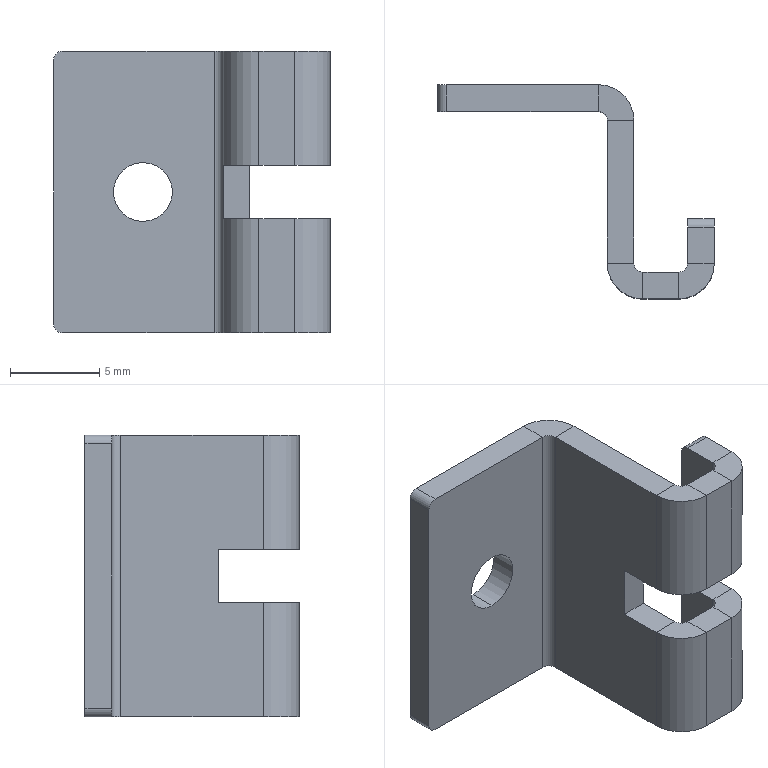Part | SolidWorks | features Fillet 1, FlatPattern 1, HoleWzd 1, ICE 1, SMBaseFlange 1, SheetMetal 1 | 1 solid | 58 faces | box 15.5 x 12 x 15.8 mm | volume 586.671 mm3 | plane 40 | cylinder 18 | commonest cylinder face diameters 1 x11 4 x5 3.3 x2
STEP:
#1=CARTESIAN_POINT('',(5.,-1.5,-1.65));
#2=VERTEX_POINT('',#1);
#3=CARTESIAN_POINT('',(5.,-1.5,1.65));
#4=VERTEX_POINT('',#3);
#5=CARTESIAN_POINT('',(5.,-1.5,0.));
#6=DIRECTION('',(0.,1.,0.));
#7=DIRECTION('',(0.,0.,1.));
#8=AXIS2_PLACEMENT_3D('',#5,#6,#7);
#9=CIRCLE('',#8,1.65);
#10=EDGE_CURVE('',#2,#4,#9,.T.);
#11=ORIENTED_EDGE('',*,*,#10,.F.);
#12=CARTESIAN_POINT('',(5.,0.,-1.65));
#13=VERTEX_POINT('',#12);
#14=CARTESIAN_POINT('',(5.,0.,-1.65));
#15=DIRECTION('',(0.,1.,0.));
#16=VECTOR('',#15,1000.);
#17=LINE('',#14,#16);
#18=EDGE_CURVE('',#2,#13,#17,.T.);
#19=ORIENTED_EDGE('',*,*,#18,.T.);
#20=CARTESIAN_POINT('',(5.,0.,1.65));
#21=VERTEX_POINT('',#20);
#22=CARTESIAN_POINT('',(5.,0.,0.));
#23=DIRECTION('',(0.,1.,0.));
#24=DIRECTION('',(0.,0.,1.));
#25=AXIS2_PLACEMENT_3D('',#22,#23,#24);
#26=CIRCLE('',#25,1.65);
#27=EDGE_CURVE('',#13,#21,#26,.T.);
#28=ORIENTED_EDGE('',*,*,#27,.T.);
#29=CARTESIAN_POINT('',(5.,0.,1.65));
#30=DIRECTION('',(0.,1.,0.));
#31=VECTOR('',#30,1000.);
#32=LINE('',#29,#31);
#33=EDGE_CURVE('',#4,#21,#32,.T.);
#34=ORIENTED_EDGE('',*,*,#33,.F.);
#35=EDGE_LOOP('',(#11,#19,#28,#34));
#36=FACE_OUTER_BOUND('',#35,.T.);
#37=CARTESIAN_POINT('',(5.,0.,0.));
#38=DIRECTION('',(0.,1.,0.));
#39=DIRECTION('',(0.,0.,1.));
#40=AXIS2_PLACEMENT_3D('',#37,#38,#39);
#41=CYLINDRICAL_SURFACE('',#40,1.65);
#42=ADVANCED_FACE('',(#36),#41,.F.);
#43=CARTESIAN_POINT('',(11.,-7.5,1.5));
#44=VERTEX_POINT('',#43);
#45=CARTESIAN_POINT('',(11.,-10.,1.5));
#46=VERTEX_POINT('',#45);
#47=CARTESIAN_POINT('',(11.,0.,1.5));
#48=DIRECTION('',(0.,-1.,0.));
#49=VECTOR('',#48,1000.);
#50=LINE('',#47,#49);
#51=EDGE_CURVE('',#44,#46,#50,.T.);
#52=ORIENTED_EDGE('',*,*,#51,.T.);
#53=CARTESIAN_POINT('',(9.5,-10.,1.5));
#54=VERTEX_POINT('',#53);
#55=CARTESIAN_POINT('',(11.,-10.,1.5));
#56=DIRECTION('',(-1.,0.,0.));
#57=VECTOR('',#56,1000.);
#58=LINE('',#55,#57);
#59=EDGE_CURVE('',#46,#54,#58,.T.);
#60=ORIENTED_EDGE('',*,*,#59,.T.);
#61=CARTESIAN_POINT('',(9.5,-7.5,1.5));
#62=VERTEX_POINT('',#61);
#63=CARTESIAN_POINT('',(9.5,0.,1.5));
#64=DIRECTION('',(0.,-1.,0.));
#65=VECTOR('',#64,1000.);
#66=LINE('',#63,#65);
#67=EDGE_CURVE('',#62,#54,#66,.T.);
#68=ORIENTED_EDGE('',*,*,#67,.F.);
#69=CARTESIAN_POINT('',(0.,-7.5,1.5));
#70=DIRECTION('',(1.,0.,0.));
#71=VECTOR('',#70,1000.);
#72=LINE('',#69,#71);
#73=EDGE_CURVE('',#62,#44,#72,.T.);
#74=ORIENTED_EDGE('',*,*,#73,.T.);
#75=EDGE_LOOP('',(#52,#60,#68,#74));
#76=FACE_OUTER_BOUND('',#75,.T.);
#77=CARTESIAN_POINT('',(0.,-7.5,1.5));
#78=DIRECTION('',(0.,0.,1.));
#79=DIRECTION('',(0.,-1.,0.));
#80=AXIS2_PLACEMENT_3D('',#77,#78,#79);
#81=PLANE('',#80);
#82=ADVANCED_FACE('',(#76),#81,.F.);
#83=CARTESIAN_POINT('',(11.5,-12.,1.5));
#84=VERTEX_POINT('',#83);
#85=CARTESIAN_POINT('',(13.5,-12.,1.5));
#86=VERTEX_POINT('',#85);
#87=CARTESIAN_POINT('',(0.,-12.,1.5));
#88=DIRECTION('',(1.,0.,0.));
#89=VECTOR('',#88,1000.);
#90=LINE('',#87,#89);
#91=EDGE_CURVE('',#84,#86,#90,.T.);
#92=ORIENTED_EDGE('',*,*,#91,.F.);
#93=CARTESIAN_POINT('',(11.5,-10.5,1.5));
#94=VERTEX_POINT('',#93);
#95=CARTESIAN_POINT('',(11.5,-12.,1.5));
#96=DIRECTION('',(0.,1.,0.));
#97=VECTOR('',#96,1000.);
#98=LINE('',#95,#97);
#99=EDGE_CURVE('',#84,#94,#98,.T.);
#100=ORIENTED_EDGE('',*,*,#99,.T.);
#101=CARTESIAN_POINT('',(13.5,-10.5,1.5));
#102=VERTEX_POINT('',#101);
#103=CARTESIAN_POINT('',(11.,-10.5,1.5));
#104=DIRECTION('',(1.,0.,0.));
#105=VECTOR('',#104,1000.);
#106=LINE('',#103,#105);
#107=EDGE_CURVE('',#94,#102,#106,.T.);
#108=ORIENTED_EDGE('',*,*,#107,.T.);
#109=CARTESIAN_POINT('',(13.5,-10.5,1.5));
#110=DIRECTION('',(0.,-1.,0.));
#111=VECTOR('',#110,1000.);
#112=LINE('',#109,#111);
#113=EDGE_CURVE('',#102,#86,#112,.T.);
#114=ORIENTED_EDGE('',*,*,#113,.T.);
#115=EDGE_LOOP('',(#92,#100,#108,#114));
#116=FACE_OUTER_BOUND('',#115,.T.);
#117=CARTESIAN_POINT('',(0.,-7.5,1.5));
#118=DIRECTION('',(0.,0.,1.));
#119=DIRECTION('',(0.,-1.,0.));
#120=AXIS2_PLACEMENT_3D('',#117,#118,#119);
#121=PLANE('',#120);
#122=ADVANCED_FACE('',(#116),#121,.F.);
#123=ORIENTED_EDGE('',*,*,#59,.F.);
#124=CARTESIAN_POINT('',(11.5,-10.,1.5));
#125=DIRECTION('',(0.,0.,1.));
#126=DIRECTION('',(0.,-1.,0.));
#127=AXIS2_PLACEMENT_3D('',#124,#125,#126);
#128=CIRCLE('',#127,0.5);
#129=EDGE_CURVE('',#46,#94,#128,.T.);
#130=ORIENTED_EDGE('',*,*,#129,.T.);
#131=ORIENTED_EDGE('',*,*,#99,.F.);
#132=CARTESIAN_POINT('',(11.5,-10.,1.5));
#133=DIRECTION('',(0.,0.,1.));
#134=DIRECTION('',(0.,-1.,0.));
#135=AXIS2_PLACEMENT_3D('',#132,#133,#134);
#136=CIRCLE('',#135,2.);
#137=EDGE_CURVE('',#54,#84,#136,.T.);
#138=ORIENTED_EDGE('',*,*,#137,.F.);
#139=EDGE_LOOP('',(#123,#130,#131,#138));
#140=FACE_OUTER_BOUND('',#139,.T.);
#141=CARTESIAN_POINT('',(0.,-7.5,1.5));
#142=DIRECTION('',(0.,0.,1.));
#143=DIRECTION('',(0.,-1.,0.));
#144=AXIS2_PLACEMENT_3D('',#141,#142,#143);
#145=PLANE('',#144);
#146=ADVANCED_FACE('',(#140),#145,.F.);
#147=CARTESIAN_POINT('',(14.,-10.,1.5));
#148=VERTEX_POINT('',#147);
#149=CARTESIAN_POINT('',(14.,-8.,1.5));
#150=VERTEX_POINT('',#149);
#151=CARTESIAN_POINT('',(14.,-10.5,1.5));
#152=DIRECTION('',(0.,1.,0.));
#153=VECTOR('',#152,1000.);
#154=LINE('',#151,#153);
#155=EDGE_CURVE('',#148,#150,#154,.T.);
#156=ORIENTED_EDGE('',*,*,#155,.T.);
#157=CARTESIAN_POINT('',(15.5,-8.,1.5));
#158=VERTEX_POINT('',#157);
#159=CARTESIAN_POINT('',(15.5,-8.,1.5));
#160=DIRECTION('',(1.,0.,0.));
#161=VECTOR('',#160,1000.);
#162=LINE('',#159,#161);
#163=EDGE_CURVE('',#150,#158,#162,.T.);
#164=ORIENTED_EDGE('',*,*,#163,.T.);
#165=CARTESIAN_POINT('',(15.5,-10.,1.5));
#166=VERTEX_POINT('',#165);
#167=CARTESIAN_POINT('',(15.5,-7.5,1.5));
#168=DIRECTION('',(0.,-1.,0.));
#169=VECTOR('',#168,1000.);
#170=LINE('',#167,#169);
#171=EDGE_CURVE('',#158,#166,#170,.T.);
#172=ORIENTED_EDGE('',*,*,#171,.T.);
#173=CARTESIAN_POINT('',(15.5,-10.,1.5));
#174=DIRECTION('',(-1.,0.,0.));
#175=VECTOR('',#174,1000.);
#176=LINE('',#173,#175);
#177=EDGE_CURVE('',#166,#148,#176,.T.);
#178=ORIENTED_EDGE('',*,*,#177,.T.);
#179=EDGE_LOOP('',(#156,#164,#172,#178));
#180=FACE_OUTER_BOUND('',#179,.T.);
#181=CARTESIAN_POINT('',(0.,-7.5,1.5));
#182=DIRECTION('',(0.,0.,1.));
#183=DIRECTION('',(0.,-1.,0.));
#184=AXIS2_PLACEMENT_3D('',#181,#182,#183);
#185=PLANE('',#184);
#186=ADVANCED_FACE('',(#180),#185,.F.);
#187=CARTESIAN_POINT('',(9.5,-10.,-1.5));
#188=VERTEX_POINT('',#187);
#189=CARTESIAN_POINT('',(9.5,-7.5,-1.5));
#190=VERTEX_POINT('',#189);
#191=CARTESIAN_POINT('',(9.5,0.,-1.5));
#192=DIRECTION('',(0.,1.,0.));
#193=VECTOR('',#192,1000.);
#194=LINE('',#191,#193);
#195=EDGE_CURVE('',#188,#190,#194,.T.);
#196=ORIENTED_EDGE('',*,*,#195,.F.);
#197=CARTESIAN_POINT('',(11.,-10.,-1.5));
#198=VERTEX_POINT('',#197);
#199=CARTESIAN_POINT('',(9.5,-10.,-1.5));
#200=DIRECTION('',(1.,0.,0.));
#201=VECTOR('',#200,1000.);
#202=LINE('',#199,#201);
#203=EDGE_CURVE('',#188,#198,#202,.T.);
#204=ORIENTED_EDGE('',*,*,#203,.T.);
#205=CARTESIAN_POINT('',(11.,-7.5,-1.5));
#206=VERTEX_POINT('',#205);
#207=CARTESIAN_POINT('',(11.,0.,-1.5));
#208=DIRECTION('',(0.,1.,0.));
#209=VECTOR('',#208,1000.);
#210=LINE('',#207,#209);
#211=EDGE_CURVE('',#198,#206,#210,.T.);
#212=ORIENTED_EDGE('',*,*,#211,.T.);
#213=CARTESIAN_POINT('',(0.,-7.5,-1.5));
#214=DIRECTION('',(1.,0.,0.));
#215=VECTOR('',#214,1000.);
#216=LINE('',#213,#215);
#217=EDGE_CURVE('',#190,#206,#216,.T.);
#218=ORIENTED_EDGE('',*,*,#217,.F.);
#219=EDGE_LOOP('',(#196,#204,#212,#218));
#220=FACE_OUTER_BOUND('',#219,.T.);
#221=CARTESIAN_POINT('',(0.,-7.5,-1.5));
#222=DIRECTION('',(0.,0.,-1.));
#223=DIRECTION('',(0.,1.,0.));
#224=AXIS2_PLACEMENT_3D('',#221,#222,#223);
#225=PLANE('',#224);
#226=ADVANCED_FACE('',(#220),#225,.F.);
#227=CARTESIAN_POINT('',(13.5,-10.5,-1.5));
#228=VERTEX_POINT('',#227);
#229=CARTESIAN_POINT('',(11.5,-10.5,-1.5));
#230=VERTEX_POINT('',#229);
#231=CARTESIAN_POINT('',(11.,-10.5,-1.5));
#232=DIRECTION('',(-1.,0.,0.));
#233=VECTOR('',#232,1000.);
#234=LINE('',#231,#233);
#235=EDGE_CURVE('',#228,#230,#234,.T.);
#236=ORIENTED_EDGE('',*,*,#235,.T.);
#237=CARTESIAN_POINT('',(11.5,-12.,-1.5));
#238=VERTEX_POINT('',#237);
#239=CARTESIAN_POINT('',(11.5,-10.5,-1.5));
#240=DIRECTION('',(0.,-1.,0.));
#241=VECTOR('',#240,1000.);
#242=LINE('',#239,#241);
#243=EDGE_CURVE('',#230,#238,#242,.T.);
#244=ORIENTED_EDGE('',*,*,#243,.T.);
#245=CARTESIAN_POINT('',(13.5,-12.,-1.5));
#246=VERTEX_POINT('',#245);
#247=CARTESIAN_POINT('',(0.,-12.,-1.5));
#248=DIRECTION('',(1.,0.,0.));
#249=VECTOR('',#248,1000.);
#250=LINE('',#247,#249);
#251=EDGE_CURVE('',#238,#246,#250,.T.);
#252=ORIENTED_EDGE('',*,*,#251,.T.);
#253=CARTESIAN_POINT('',(13.5,-12.,-1.5));
#254=DIRECTION('',(0.,1.,0.));
#255=VECTOR('',#254,1000.);
#256=LINE('',#253,#255);
#257=EDGE_CURVE('',#246,#228,#256,.T.);
#258=ORIENTED_EDGE('',*,*,#257,.T.);
#259=EDGE_LOOP('',(#236,#244,#252,#258));
#260=FACE_OUTER_BOUND('',#259,.T.);
#261=CARTESIAN_POINT('',(0.,-7.5,-1.5));
#262=DIRECTION('',(0.,0.,-1.));
#263=DIRECTION('',(0.,1.,0.));
#264=AXIS2_PLACEMENT_3D('',#261,#262,#263);
#265=PLANE('',#264);
#266=ADVANCED_FACE('',(#260),#265,.F.);
#267=ORIENTED_EDGE('',*,*,#203,.F.);
#268=CARTESIAN_POINT('',(11.5,-10.,-1.5));
#269=DIRECTION('',(0.,0.,-1.));
#270=DIRECTION('',(0.,1.,0.));
#271=AXIS2_PLACEMENT_3D('',#268,#269,#270);
#272=CIRCLE('',#271,2.);
#273=EDGE_CURVE('',#238,#188,#272,.T.);
#274=ORIENTED_EDGE('',*,*,#273,.F.);
#275=ORIENTED_EDGE('',*,*,#243,.F.);
#276=CARTESIAN_POINT('',(11.5,-10.,-1.5));
#277=DIRECTION('',(0.,0.,-1.));
#278=DIRECTION('',(0.,1.,0.));
#279=AXIS2_PLACEMENT_3D('',#276,#277,#278);
#280=CIRCLE('',#279,0.5);
#281=EDGE_CURVE('',#230,#198,#280,.T.);
#282=ORIENTED_EDGE('',*,*,#281,.T.);
#283=EDGE_LOOP('',(#267,#274,#275,#282));
#284=FACE_OUTER_BOUND('',#283,.T.);
#285=CARTESIAN_POINT('',(0.,-7.5,-1.5));
#286=DIRECTION('',(0.,0.,-1.));
#287=DIRECTION('',(0.,1.,0.));
#288=AXIS2_PLACEMENT_3D('',#285,#286,#287);
#289=PLANE('',#288);
#290=ADVANCED_FACE('',(#284),#289,.F.);
#291=CARTESIAN_POINT('',(15.5,-10.,-1.5));
#292=VERTEX_POINT('',#291);
#293=CARTESIAN_POINT('',(15.5,-8.,-1.5));
#294=VERTEX_POINT('',#293);
#295=CARTESIAN_POINT('',(15.5,-7.5,-1.5));
#296=DIRECTION('',(0.,1.,0.));
#297=VECTOR('',#296,1000.);
#298=LINE('',#295,#297);
#299=EDGE_CURVE('',#292,#294,#298,.T.);
#300=ORIENTED_EDGE('',*,*,#299,.T.);
#301=CARTESIAN_POINT('',(14.,-8.,-1.5));
#302=VERTEX_POINT('',#301);
#303=CARTESIAN_POINT('',(14.,-8.,-1.5));
#304=DIRECTION('',(-1.,0.,0.));
#305=VECTOR('',#304,1000.);
#306=LINE('',#303,#305);
#307=EDGE_CURVE('',#294,#302,#306,.T.);
#308=ORIENTED_EDGE('',*,*,#307,.T.);
#309=CARTESIAN_POINT('',(14.,-10.,-1.5));
#310=VERTEX_POINT('',#309);
#311=CARTESIAN_POINT('',(14.,-10.5,-1.5));
#312=DIRECTION('',(0.,-1.,0.));
#313=VECTOR('',#312,1000.);
#314=LINE('',#311,#313);
#315=EDGE_CURVE('',#302,#310,#314,.T.);
#316=ORIENTED_EDGE('',*,*,#315,.T.);
#317=CARTESIAN_POINT('',(14.,-10.,-1.5));
#318=DIRECTION('',(1.,0.,0.));
#319=VECTOR('',#318,1000.);
#320=LINE('',#317,#319);
#321=EDGE_CURVE('',#310,#292,#320,.T.);
#322=ORIENTED_EDGE('',*,*,#321,.T.);
#323=EDGE_LOOP('',(#300,#308,#316,#322));
#324=FACE_OUTER_BOUND('',#323,.T.);
#325=CARTESIAN_POINT('',(0.,-7.5,-1.5));
#326=DIRECTION('',(0.,0.,-1.));
#327=DIRECTION('',(0.,1.,0.));
#328=AXIS2_PLACEMENT_3D('',#325,#326,#327);
#329=PLANE('',#328);
#330=ADVANCED_FACE('',(#324),#329,.F.);
#331=CARTESIAN_POINT('',(15.5,-10.,-7.9));
#332=VERTEX_POINT('',#331);
#333=CARTESIAN_POINT('',(15.5,-8.,-7.9));
#334=VERTEX_POINT('',#333);
#335=CARTESIAN_POINT('',(15.5,-10.5,-7.9));
#336=DIRECTION('',(0.,1.,0.));
#337=VECTOR('',#336,1000.);
#338=LINE('',#335,#337);
#339=EDGE_CURVE('',#332,#334,#338,.T.);
#340=ORIENTED_EDGE('',*,*,#339,.T.);
#341=CARTESIAN_POINT('',(15.5,-7.5,-7.4));
#342=VERTEX_POINT('',#341);
#343=CARTESIAN_POINT('',(15.5,-8.,-7.4));
#344=DIRECTION('',(1.,0.,0.));
#345=DIRECTION('',(0.,0.,1.));
#346=AXIS2_PLACEMENT_3D('',#343,#344,#345);
#347=CIRCLE('',#346,0.5);
#348=EDGE_CURVE('',#334,#342,#347,.T.);
#349=ORIENTED_EDGE('',*,*,#348,.T.);
#350=CARTESIAN_POINT('',(15.5,-7.5,-2.));
#351=VERTEX_POINT('',#350);
#352=CARTESIAN_POINT('',(15.5,-7.5,7.9));
#353=DIRECTION('',(0.,0.,-1.));
#354=VECTOR('',#353,1000.);
#355=LINE('',#352,#354);
#356=EDGE_CURVE('',#351,#342,#355,.T.);
#357=ORIENTED_EDGE('',*,*,#356,.F.);
#358=CARTESIAN_POINT('',(15.5,-8.,-2.));
#359=DIRECTION('',(1.,0.,0.));
#360=DIRECTION('',(0.,0.,1.));
#361=AXIS2_PLACEMENT_3D('',#358,#359,#360);
#362=CIRCLE('',#361,0.5);
#363=EDGE_CURVE('',#351,#294,#362,.T.);
#364=ORIENTED_EDGE('',*,*,#363,.T.);
#365=ORIENTED_EDGE('',*,*,#299,.F.);
#366=CARTESIAN_POINT('',(15.5,-10.,7.9));
#367=DIRECTION('',(0.,0.,-1.));
#368=VECTOR('',#367,1000.);
#369=LINE('',#366,#368);
#370=EDGE_CURVE('',#292,#332,#369,.T.);
#371=ORIENTED_EDGE('',*,*,#370,.T.);
#372=EDGE_LOOP('',(#340,#349,#357,#364,#365,#371));
#373=FACE_OUTER_BOUND('',#372,.T.);
#374=CARTESIAN_POINT('',(15.5,-10.5,7.9));
#375=DIRECTION('',(-1.,0.,0.));
#376=DIRECTION('',(0.,0.,1.));
#377=AXIS2_PLACEMENT_3D('',#374,#375,#376);
#378=PLANE('',#377);
#379=ADVANCED_FACE('',(#373),#378,.F.);
#380=ORIENTED_EDGE('',*,*,#356,.T.);
#381=CARTESIAN_POINT('',(14.,-7.5,-7.4));
#382=VERTEX_POINT('',#381);
#383=CARTESIAN_POINT('',(14.,-7.5,-7.4));
#384=DIRECTION('',(-1.,0.,0.));
#385=VECTOR('',#384,1000.);
#386=LINE('',#383,#385);
#387=EDGE_CURVE('',#342,#382,#386,.T.);
#388=ORIENTED_EDGE('',*,*,#387,.T.);
#389=CARTESIAN_POINT('',(14.,-7.5,-2.));
#390=VERTEX_POINT('',#389);
#391=CARTESIAN_POINT('',(14.,-7.5,7.9));
#392=DIRECTION('',(0.,0.,-1.));
#393=VECTOR('',#392,1000.);
#394=LINE('',#391,#393);
#395=EDGE_CURVE('',#390,#382,#394,.T.);
#396=ORIENTED_EDGE('',*,*,#395,.F.);
#397=CARTESIAN_POINT('',(15.5,-7.5,-2.));
#398=DIRECTION('',(1.,0.,0.));
#399=VECTOR('',#398,1000.);
#400=LINE('',#397,#399);
#401=EDGE_CURVE('',#390,#351,#400,.T.);
#402=ORIENTED_EDGE('',*,*,#401,.T.);
#403=EDGE_LOOP('',(#380,#388,#396,#402));
#404=FACE_OUTER_BOUND('',#403,.T.);
#405=CARTESIAN_POINT('',(14.,-7.5,7.9));
#406=DIRECTION('',(0.,1.,0.));
#407=DIRECTION('',(0.,0.,1.));
#408=AXIS2_PLACEMENT_3D('',#405,#406,#407);
#409=PLANE('',#408);
#410=ADVANCED_FACE('',(#404),#409,.T.);
#411=ORIENTED_EDGE('',*,*,#395,.T.);
#412=CARTESIAN_POINT('',(14.,-8.,-7.9));
#413=VERTEX_POINT('',#412);
#414=CARTESIAN_POINT('',(14.,-8.,-7.4));
#415=DIRECTION('',(-1.,0.,0.));
#416=DIRECTION('',(0.,0.,1.));
#417=AXIS2_PLACEMENT_3D('',#414,#415,#416);
#418=CIRCLE('',#417,0.5);
#419=EDGE_CURVE('',#382,#413,#418,.T.);
#420=ORIENTED_EDGE('',*,*,#419,.T.);
#421=CARTESIAN_POINT('',(14.,-10.,-7.9));
#422=VERTEX_POINT('',#421);
#423=CARTESIAN_POINT('',(14.,-10.5,-7.9));
#424=DIRECTION('',(0.,1.,0.));
#425=VECTOR('',#424,1000.);
#426=LINE('',#423,#425);
#427=EDGE_CURVE('',#422,#413,#426,.T.);
#428=ORIENTED_EDGE('',*,*,#427,.F.);
#429=CARTESIAN_POINT('',(14.,-10.,7.9));
#430=DIRECTION('',(0.,0.,-1.));
#431=VECTOR('',#430,1000.);
#432=LINE('',#429,#431);
#433=EDGE_CURVE('',#310,#422,#432,.T.);
#434=ORIENTED_EDGE('',*,*,#433,.F.);
#435=ORIENTED_EDGE('',*,*,#315,.F.);
#436=CARTESIAN_POINT('',(14.,-8.,-2.));
#437=DIRECTION('',(-1.,0.,0.));
#438=DIRECTION('',(0.,0.,1.));
#439=AXIS2_PLACEMENT_3D('',#436,#437,#438);
#440=CIRCLE('',#439,0.5);
#441=EDGE_CURVE('',#302,#390,#440,.T.);
#442=ORIENTED_EDGE('',*,*,#441,.T.);
#443=EDGE_LOOP('',(#411,#420,#428,#434,#435,#442));
#444=FACE_OUTER_BOUND('',#443,.T.);
#445=CARTESIAN_POINT('',(14.,-10.5,7.9));
#446=DIRECTION('',(-1.,0.,0.));
#447=DIRECTION('',(0.,0.,1.));
#448=AXIS2_PLACEMENT_3D('',#445,#446,#447);
#449=PLANE('',#448);
#450=ADVANCED_FACE('',(#444),#449,.T.);
#451=CARTESIAN_POINT('',(13.5,-10.,-1.5));
#452=DIRECTION('',(0.,0.,-1.));
#453=DIRECTION('',(0.,1.,0.));
#454=AXIS2_PLACEMENT_3D('',#451,#452,#453);
#455=CIRCLE('',#454,0.5);
#456=EDGE_CURVE('',#310,#228,#455,.T.);
#457=ORIENTED_EDGE('',*,*,#456,.F.);
#458=ORIENTED_EDGE('',*,*,#433,.T.);
#459=CARTESIAN_POINT('',(13.5,-10.5,-7.9));
#460=VERTEX_POINT('',#459);
#461=CARTESIAN_POINT('',(13.5,-10.,-7.9));
#462=DIRECTION('',(0.,0.,1.));
#463=DIRECTION('',(-1.,0.,0.));
#464=AXIS2_PLACEMENT_3D('',#461,#462,#463);
#465=CIRCLE('',#464,0.5);
#466=EDGE_CURVE('',#460,#422,#465,.T.);
#467=ORIENTED_EDGE('',*,*,#466,.F.);
#468=CARTESIAN_POINT('',(13.5,-10.5,7.9));
#469=DIRECTION('',(0.,0.,-1.));
#470=VECTOR('',#469,1000.);
#471=LINE('',#468,#470);
#472=EDGE_CURVE('',#228,#460,#471,.T.);
#473=ORIENTED_EDGE('',*,*,#472,.F.);
#474=EDGE_LOOP('',(#457,#458,#467,#473));
#475=FACE_OUTER_BOUND('',#474,.T.);
#476=CARTESIAN_POINT('',(13.5,-10.,7.9));
#477=DIRECTION('',(0.,0.,-1.));
#478=DIRECTION('',(-1.,0.,0.));
#479=AXIS2_PLACEMENT_3D('',#476,#477,#478);
#480=CYLINDRICAL_SURFACE('',#479,0.5);
#481=ADVANCED_FACE('',(#475),#480,.F.);
#482=ORIENTED_EDGE('',*,*,#235,.F.);
#483=ORIENTED_EDGE('',*,*,#472,.T.);
#484=CARTESIAN_POINT('',(11.5,-10.5,-7.9));
#485=VERTEX_POINT('',#484);
#486=CARTESIAN_POINT('',(11.,-10.5,-7.9));
#487=DIRECTION('',(1.,0.,0.));
#488=VECTOR('',#487,1000.);
#489=LINE('',#486,#488);
#490=EDGE_CURVE('',#485,#460,#489,.T.);
#491=ORIENTED_EDGE('',*,*,#490,.F.);
#492=CARTESIAN_POINT('',(11.5,-10.5,7.9));
#493=DIRECTION('',(0.,0.,-1.));
#494=VECTOR('',#493,1000.);
#495=LINE('',#492,#494);
#496=EDGE_CURVE('',#230,#485,#495,.T.);
#497=ORIENTED_EDGE('',*,*,#496,.F.);
#498=EDGE_LOOP('',(#482,#483,#491,#497));
#499=FACE_OUTER_BOUND('',#498,.T.);
#500=CARTESIAN_POINT('',(11.,-10.5,7.9));
#501=DIRECTION('',(0.,1.,0.));
#502=DIRECTION('',(0.,0.,1.));
#503=AXIS2_PLACEMENT_3D('',#500,#501,#502);
#504=PLANE('',#503);
#505=ADVANCED_FACE('',(#499),#504,.T.);
#506=ORIENTED_EDGE('',*,*,#281,.F.);
#507=ORIENTED_EDGE('',*,*,#496,.T.);
#508=CARTESIAN_POINT('',(11.,-10.,-7.9));
#509=VERTEX_POINT('',#508);
#510=CARTESIAN_POINT('',(11.5,-10.,-7.9));
#511=DIRECTION('',(0.,0.,1.));
#512=DIRECTION('',(-1.,0.,0.));
#513=AXIS2_PLACEMENT_3D('',#510,#511,#512);
#514=CIRCLE('',#513,0.5);
#515=EDGE_CURVE('',#509,#485,#514,.T.);
#516=ORIENTED_EDGE('',*,*,#515,.F.);
#517=CARTESIAN_POINT('',(11.,-10.,7.9));
#518=DIRECTION('',(0.,0.,-1.));
#519=VECTOR('',#518,1000.);
#520=LINE('',#517,#519);
#521=EDGE_CURVE('',#198,#509,#520,.T.);
#522=ORIENTED_EDGE('',*,*,#521,.F.);
#523=EDGE_LOOP('',(#506,#507,#516,#522));
#524=FACE_OUTER_BOUND('',#523,.T.);
#525=CARTESIAN_POINT('',(11.5,-10.,7.9));
#526=DIRECTION('',(0.,0.,-1.));
#527=DIRECTION('',(-1.,0.,0.));
#528=AXIS2_PLACEMENT_3D('',#525,#526,#527);
#529=CYLINDRICAL_SURFACE('',#528,0.5);
#530=ADVANCED_FACE('',(#524),#529,.F.);
#531=CARTESIAN_POINT('',(11.5,-12.,-7.9));
#532=VERTEX_POINT('',#531);
#533=CARTESIAN_POINT('',(11.5,-12.,7.9));
#534=DIRECTION('',(0.,0.,-1.));
#535=VECTOR('',#534,1000.);
#536=LINE('',#533,#535);
#537=EDGE_CURVE('',#238,#532,#536,.T.);
#538=ORIENTED_EDGE('',*,*,#537,.F.);
#539=ORIENTED_EDGE('',*,*,#273,.T.);
#540=CARTESIAN_POINT('',(9.5,-10.,-7.9));
#541=VERTEX_POINT('',#540);
#542=CARTESIAN_POINT('',(9.5,-10.,7.9));
#543=DIRECTION('',(0.,0.,-1.));
#544=VECTOR('',#543,1000.);
#545=LINE('',#542,#544);
#546=EDGE_CURVE('',#188,#541,#545,.T.);
#547=ORIENTED_EDGE('',*,*,#546,.T.);
#548=CARTESIAN_POINT('',(11.5,-10.,-7.9));
#549=DIRECTION('',(0.,0.,1.));
#550=DIRECTION('',(1.,0.,0.));
#551=AXIS2_PLACEMENT_3D('',#548,#549,#550);
#552=CIRCLE('',#551,2.);
#553=EDGE_CURVE('',#541,#532,#552,.T.);
#554=ORIENTED_EDGE('',*,*,#553,.T.);
#555=EDGE_LOOP('',(#538,#539,#547,#554));
#556=FACE_OUTER_BOUND('',#555,.T.);
#557=CARTESIAN_POINT('',(11.5,-10.,7.9));
#558=DIRECTION('',(0.,0.,-1.));
#559=DIRECTION('',(-1.,0.,0.));
#560=AXIS2_PLACEMENT_3D('',#557,#558,#559);
#561=CYLINDRICAL_SURFACE('',#560,2.);
#562=ADVANCED_FACE('',(#556),#561,.T.);
#563=CARTESIAN_POINT('',(13.5,-12.,-7.9));
#564=VERTEX_POINT('',#563);
#565=CARTESIAN_POINT('',(13.5,-12.,7.9));
#566=DIRECTION('',(0.,0.,-1.));
#567=VECTOR('',#566,1000.);
#568=LINE('',#565,#567);
#569=EDGE_CURVE('',#246,#564,#568,.T.);
#570=ORIENTED_EDGE('',*,*,#569,.F.);
#571=ORIENTED_EDGE('',*,*,#251,.F.);
#572=ORIENTED_EDGE('',*,*,#537,.T.);
#573=CARTESIAN_POINT('',(11.,-12.,-7.9));
#574=DIRECTION('',(1.,0.,0.));
#575=VECTOR('',#574,1000.);
#576=LINE('',#573,#575);
#577=EDGE_CURVE('',#532,#564,#576,.T.);
#578=ORIENTED_EDGE('',*,*,#577,.T.);
#579=EDGE_LOOP('',(#570,#571,#572,#578));
#580=FACE_OUTER_BOUND('',#579,.T.);
#581=CARTESIAN_POINT('',(11.,-12.,7.9));
#582=DIRECTION('',(0.,1.,0.));
#583=DIRECTION('',(0.,0.,1.));
#584=AXIS2_PLACEMENT_3D('',#581,#582,#583);
#585=PLANE('',#584);
#586=ADVANCED_FACE('',(#580),#585,.F.);
#587=ORIENTED_EDGE('',*,*,#370,.F.);
#588=CARTESIAN_POINT('',(13.5,-10.,-1.5));
#589=DIRECTION('',(0.,0.,-1.));
#590=DIRECTION('',(0.,1.,0.));
#591=AXIS2_PLACEMENT_3D('',#588,#589,#590);
#592=CIRCLE('',#591,2.);
#593=EDGE_CURVE('',#292,#246,#592,.T.);
#594=ORIENTED_EDGE('',*,*,#593,.T.);
#595=ORIENTED_EDGE('',*,*,#569,.T.);
#596=CARTESIAN_POINT('',(13.5,-10.,-7.9));
#597=DIRECTION('',(0.,0.,1.));
#598=DIRECTION('',(1.,0.,0.));
#599=AXIS2_PLACEMENT_3D('',#596,#597,#598);
#600=CIRCLE('',#599,2.);
#601=EDGE_CURVE('',#564,#332,#600,.T.);
#602=ORIENTED_EDGE('',*,*,#601,.T.);
#603=EDGE_LOOP('',(#587,#594,#595,#602));
#604=FACE_OUTER_BOUND('',#603,.T.);
#605=CARTESIAN_POINT('',(13.5,-10.,7.9));
#606=DIRECTION('',(0.,0.,-1.));
#607=DIRECTION('',(-1.,0.,0.));
#608=AXIS2_PLACEMENT_3D('',#605,#606,#607);
#609=CYLINDRICAL_SURFACE('',#608,2.);
#610=ADVANCED_FACE('',(#604),#609,.T.);
#611=CARTESIAN_POINT('',(11.,-2.,7.9));
#612=VERTEX_POINT('',#611);
#613=CARTESIAN_POINT('',(9.5,-2.,7.9));
#614=VERTEX_POINT('',#613);
#615=CARTESIAN_POINT('',(11.,-2.,7.9));
#616=DIRECTION('',(-1.,0.,0.));
#617=VECTOR('',#616,1000.);
#618=LINE('',#615,#617);
#619=EDGE_CURVE('',#612,#614,#618,.T.);
#620=ORIENTED_EDGE('',*,*,#619,.F.);
#621=CARTESIAN_POINT('',(9.,0.,7.9));
#622=VERTEX_POINT('',#621);
#623=CARTESIAN_POINT('',(9.,-2.,7.9));
#624=DIRECTION('',(0.,0.,-1.));
#625=DIRECTION('',(1.,0.,0.));
#626=AXIS2_PLACEMENT_3D('',#623,#624,#625);
#627=CIRCLE('',#626,2.);
#628=EDGE_CURVE('',#622,#612,#627,.T.);
#629=ORIENTED_EDGE('',*,*,#628,.F.);
#630=CARTESIAN_POINT('',(9.,-1.5,7.9));
#631=VERTEX_POINT('',#630);
#632=CARTESIAN_POINT('',(9.,-1.5,7.9));
#633=DIRECTION('',(0.,1.,0.));
#634=VECTOR('',#633,1000.);
#635=LINE('',#632,#634);
#636=EDGE_CURVE('',#631,#622,#635,.T.);
#637=ORIENTED_EDGE('',*,*,#636,.F.);
#638=CARTESIAN_POINT('',(9.,-2.,7.9));
#639=DIRECTION('',(0.,0.,-1.));
#640=DIRECTION('',(1.,0.,0.));
#641=AXIS2_PLACEMENT_3D('',#638,#639,#640);
#642=CIRCLE('',#641,0.5);
#643=EDGE_CURVE('',#631,#614,#642,.T.);
#644=ORIENTED_EDGE('',*,*,#643,.T.);
#645=EDGE_LOOP('',(#620,#629,#637,#644));
#646=FACE_OUTER_BOUND('',#645,.T.);
#647=CARTESIAN_POINT('',(11.,-2.,7.9));
#648=DIRECTION('',(0.,0.,1.));
#649=DIRECTION('',(1.,0.,0.));
#650=AXIS2_PLACEMENT_3D('',#647,#648,#649);
#651=PLANE('',#650);
#652=ADVANCED_FACE('',(#646),#651,.T.);
#653=CARTESIAN_POINT('',(11.,-10.,7.9));
#654=VERTEX_POINT('',#653);
#655=CARTESIAN_POINT('',(11.,0.,7.9));
#656=DIRECTION('',(0.,-1.,0.));
#657=VECTOR('',#656,1000.);
#658=LINE('',#655,#657);
#659=EDGE_CURVE('',#612,#654,#658,.T.);
#660=ORIENTED_EDGE('',*,*,#659,.F.);
#661=ORIENTED_EDGE('',*,*,#619,.T.);
#662=CARTESIAN_POINT('',(9.5,-10.,7.9));
#663=VERTEX_POINT('',#662);
#664=CARTESIAN_POINT('',(9.5,0.,7.9));
#665=DIRECTION('',(0.,-1.,0.));
#666=VECTOR('',#665,1000.);
#667=LINE('',#664,#666);
#668=EDGE_CURVE('',#614,#663,#667,.T.);
#669=ORIENTED_EDGE('',*,*,#668,.T.);
#670=CARTESIAN_POINT('',(9.5,-10.,7.9));
#671=DIRECTION('',(1.,0.,0.));
#672=VECTOR('',#671,1000.);
#673=LINE('',#670,#672);
#674=EDGE_CURVE('',#663,#654,#673,.T.);
#675=ORIENTED_EDGE('',*,*,#674,.T.);
#676=EDGE_LOOP('',(#660,#661,#669,#675));
#677=FACE_OUTER_BOUND('',#676,.T.);
#678=CARTESIAN_POINT('',(9.,-1.5,7.9));
#679=DIRECTION('',(0.,0.,1.));
#680=DIRECTION('',(1.,0.,0.));
#681=AXIS2_PLACEMENT_3D('',#678,#679,#680);
#682=PLANE('',#681);
#683=ADVANCED_FACE('',(#677),#682,.T.);
#684=CARTESIAN_POINT('',(9.,0.,-7.9));
#685=VERTEX_POINT('',#684);
#686=CARTESIAN_POINT('',(9.,-1.5,-7.9));
#687=VERTEX_POINT('',#686);
#688=CARTESIAN_POINT('',(9.,0.,-7.9));
#689=DIRECTION('',(0.,-1.,0.));
#690=VECTOR('',#689,1000.);
#691=LINE('',#688,#690);
#692=EDGE_CURVE('',#685,#687,#691,.T.);
#693=ORIENTED_EDGE('',*,*,#692,.F.);
#694=CARTESIAN_POINT('',(11.,-2.,-7.9));
#695=VERTEX_POINT('',#694);
#696=CARTESIAN_POINT('',(9.,-2.,-7.9));
#697=DIRECTION('',(0.,0.,-1.));
#698=DIRECTION('',(1.,0.,0.));
#699=AXIS2_PLACEMENT_3D('',#696,#697,#698);
#700=CIRCLE('',#699,2.);
#701=EDGE_CURVE('',#685,#695,#700,.T.);
#702=ORIENTED_EDGE('',*,*,#701,.T.);
#703=CARTESIAN_POINT('',(9.5,-2.,-7.9));
#704=VERTEX_POINT('',#703);
#705=CARTESIAN_POINT('',(9.5,-2.,-7.9));
#706=DIRECTION('',(1.,0.,0.));
#707=VECTOR('',#706,1000.);
#708=LINE('',#705,#707);
#709=EDGE_CURVE('',#704,#695,#708,.T.);
#710=ORIENTED_EDGE('',*,*,#709,.F.);
#711=CARTESIAN_POINT('',(9.,-2.,-7.9));
#712=DIRECTION('',(0.,0.,-1.));
#713=DIRECTION('',(1.,0.,0.));
#714=AXIS2_PLACEMENT_3D('',#711,#712,#713);
#715=CIRCLE('',#714,0.5);
#716=EDGE_CURVE('',#687,#704,#715,.T.);
#717=ORIENTED_EDGE('',*,*,#716,.F.);
#718=EDGE_LOOP('',(#693,#702,#710,#717));
#719=FACE_OUTER_BOUND('',#718,.T.);
#720=CARTESIAN_POINT('',(9.,0.,-7.9));
#721=DIRECTION('',(0.,0.,-1.));
#722=DIRECTION('',(-1.,0.,0.));
#723=AXIS2_PLACEMENT_3D('',#720,#721,#722);
#724=PLANE('',#723);
#725=ADVANCED_FACE('',(#719),#724,.T.);
#726=CARTESIAN_POINT('',(0.5,-1.5,-7.9));
#727=VERTEX_POINT('',#726);
#728=CARTESIAN_POINT('',(0.,-1.5,-7.9));
#729=DIRECTION('',(1.,0.,0.));
#730=VECTOR('',#729,1000.);
#731=LINE('',#728,#730);
#732=EDGE_CURVE('',#727,#687,#731,.T.);
#733=ORIENTED_EDGE('',*,*,#732,.F.);
#734=CARTESIAN_POINT('',(0.5,0.,-7.9));
#735=VERTEX_POINT('',#734);
#736=CARTESIAN_POINT('',(0.5,-2.,-7.9));
#737=DIRECTION('',(0.,1.,0.));
#738=VECTOR('',#737,1000.);
#739=LINE('',#736,#738);
#740=EDGE_CURVE('',#727,#735,#739,.T.);
#741=ORIENTED_EDGE('',*,*,#740,.T.);
#742=CARTESIAN_POINT('',(0.,0.,-7.9));
#743=DIRECTION('',(1.,0.,0.));
#744=VECTOR('',#743,1000.);
#745=LINE('',#742,#744);
#746=EDGE_CURVE('',#735,#685,#745,.T.);
#747=ORIENTED_EDGE('',*,*,#746,.T.);
#748=ORIENTED_EDGE('',*,*,#692,.T.);
#749=EDGE_LOOP('',(#733,#741,#747,#748));
#750=FACE_OUTER_BOUND('',#749,.T.);
#751=CARTESIAN_POINT('',(9.5,-2.,-7.9));
#752=DIRECTION('',(0.,0.,-1.));
#753=DIRECTION('',(-1.,0.,0.));
#754=AXIS2_PLACEMENT_3D('',#751,#752,#753);
#755=PLANE('',#754);
#756=ADVANCED_FACE('',(#750),#755,.T.);
#757=CARTESIAN_POINT('',(11.5,-10.5,7.9));
#758=VERTEX_POINT('',#757);
#759=CARTESIAN_POINT('',(11.5,-12.,7.9));
#760=VERTEX_POINT('',#759);
#761=CARTESIAN_POINT('',(11.5,-10.5,7.9));
#762=DIRECTION('',(0.,-1.,0.));
#763=VECTOR('',#762,1000.);
#764=LINE('',#761,#763);
#765=EDGE_CURVE('',#758,#760,#764,.T.);
#766=ORIENTED_EDGE('',*,*,#765,.F.);
#767=CARTESIAN_POINT('',(11.5,-10.,7.9));
#768=DIRECTION('',(0.,0.,1.));
#769=DIRECTION('',(-1.,0.,0.));
#770=AXIS2_PLACEMENT_3D('',#767,#768,#769);
#771=CIRCLE('',#770,0.5);
#772=EDGE_CURVE('',#654,#758,#771,.T.);
#773=ORIENTED_EDGE('',*,*,#772,.F.);
#774=ORIENTED_EDGE('',*,*,#674,.F.);
#775=CARTESIAN_POINT('',(11.5,-10.,7.9));
#776=DIRECTION('',(0.,0.,1.));
#777=DIRECTION('',(1.,0.,0.));
#778=AXIS2_PLACEMENT_3D('',#775,#776,#777);
#779=CIRCLE('',#778,2.);
#780=EDGE_CURVE('',#663,#760,#779,.T.);
#781=ORIENTED_EDGE('',*,*,#780,.T.);
#782=EDGE_LOOP('',(#766,#773,#774,#781));
#783=FACE_OUTER_BOUND('',#782,.T.);
#784=CARTESIAN_POINT('',(11.5,-10.5,7.9));
#785=DIRECTION('',(0.,0.,1.));
#786=DIRECTION('',(1.,0.,0.));
#787=AXIS2_PLACEMENT_3D('',#784,#785,#786);
#788=PLANE('',#787);
#789=ADVANCED_FACE('',(#783),#788,.T.);
#790=CARTESIAN_POINT('',(13.5,-10.5,7.9));
#791=VERTEX_POINT('',#790);
#792=CARTESIAN_POINT('',(11.,-10.5,7.9));
#793=DIRECTION('',(1.,0.,0.));
#794=VECTOR('',#793,1000.);
#795=LINE('',#792,#794);
#796=EDGE_CURVE('',#758,#791,#795,.T.);
#797=ORIENTED_EDGE('',*,*,#796,.F.);
#798=ORIENTED_EDGE('',*,*,#765,.T.);
#799=CARTESIAN_POINT('',(13.5,-12.,7.9));
#800=VERTEX_POINT('',#799);
#801=CARTESIAN_POINT('',(11.,-12.,7.9));
#802=DIRECTION('',(1.,0.,0.));
#803=VECTOR('',#802,1000.);
#804=LINE('',#801,#803);
#805=EDGE_CURVE('',#760,#800,#804,.T.);
#806=ORIENTED_EDGE('',*,*,#805,.T.);
#807=CARTESIAN_POINT('',(13.5,-12.,7.9));
#808=DIRECTION('',(0.,1.,0.));
#809=VECTOR('',#808,1000.);
#810=LINE('',#807,#809);
#811=EDGE_CURVE('',#800,#791,#810,.T.);
#812=ORIENTED_EDGE('',*,*,#811,.T.);
#813=EDGE_LOOP('',(#797,#798,#806,#812));
#814=FACE_OUTER_BOUND('',#813,.T.);
#815=CARTESIAN_POINT('',(9.5,-10.,7.9));
#816=DIRECTION('',(0.,0.,1.));
#817=DIRECTION('',(1.,0.,0.));
#818=AXIS2_PLACEMENT_3D('',#815,#816,#817);
#819=PLANE('',#818);
#820=ADVANCED_FACE('',(#814),#819,.T.);
#821=CARTESIAN_POINT('',(11.,-10.,-7.9));
#822=DIRECTION('',(-1.,0.,0.));
#823=VECTOR('',#822,1000.);
#824=LINE('',#821,#823);
#825=EDGE_CURVE('',#509,#541,#824,.T.);
#826=ORIENTED_EDGE('',*,*,#825,.F.);
#827=ORIENTED_EDGE('',*,*,#515,.T.);
#828=CARTESIAN_POINT('',(11.5,-12.,-7.9));
#829=DIRECTION('',(0.,1.,0.));
#830=VECTOR('',#829,1000.);
#831=LINE('',#828,#830);
#832=EDGE_CURVE('',#532,#485,#831,.T.);
#833=ORIENTED_EDGE('',*,*,#832,.F.);
#834=ORIENTED_EDGE('',*,*,#553,.F.);
#835=EDGE_LOOP('',(#826,#827,#833,#834));
#836=FACE_OUTER_BOUND('',#835,.T.);
#837=CARTESIAN_POINT('',(11.,-10.,-7.9));
#838=DIRECTION('',(0.,0.,-1.));
#839=DIRECTION('',(-1.,0.,0.));
#840=AXIS2_PLACEMENT_3D('',#837,#838,#839);
#841=PLANE('',#840);
#842=ADVANCED_FACE('',(#836),#841,.T.);
#843=CARTESIAN_POINT('',(11.,0.,-7.9));
#844=DIRECTION('',(0.,-1.,0.));
#845=VECTOR('',#844,1000.);
#846=LINE('',#843,#845);
#847=EDGE_CURVE('',#695,#509,#846,.T.);
#848=ORIENTED_EDGE('',*,*,#847,.T.);
#849=ORIENTED_EDGE('',*,*,#825,.T.);
#850=CARTESIAN_POINT('',(9.5,0.,-7.9));
#851=DIRECTION('',(0.,-1.,0.));
#852=VECTOR('',#851,1000.);
#853=LINE('',#850,#852);
#854=EDGE_CURVE('',#704,#541,#853,.T.);
#855=ORIENTED_EDGE('',*,*,#854,.F.);
#856=ORIENTED_EDGE('',*,*,#709,.T.);
#857=EDGE_LOOP('',(#848,#849,#855,#856));
#858=FACE_OUTER_BOUND('',#857,.T.);
#859=CARTESIAN_POINT('',(11.5,-12.,-7.9));
#860=DIRECTION('',(0.,0.,-1.));
#861=DIRECTION('',(-1.,0.,0.));
#862=AXIS2_PLACEMENT_3D('',#859,#860,#861);
#863=PLANE('',#862);
#864=ADVANCED_FACE('',(#858),#863,.T.);
#865=CARTESIAN_POINT('',(14.,-10.,7.9));
#866=VERTEX_POINT('',#865);
#867=CARTESIAN_POINT('',(15.5,-10.,7.9));
#868=VERTEX_POINT('',#867);
#869=CARTESIAN_POINT('',(14.,-10.,7.9));
#870=DIRECTION('',(1.,0.,0.));
#871=VECTOR('',#870,1000.);
#872=LINE('',#869,#871);
#873=EDGE_CURVE('',#866,#868,#872,.T.);
#874=ORIENTED_EDGE('',*,*,#873,.F.);
#875=CARTESIAN_POINT('',(13.5,-10.,7.9));
#876=DIRECTION('',(0.,0.,1.));
#877=DIRECTION('',(-1.,0.,0.));
#878=AXIS2_PLACEMENT_3D('',#875,#876,#877);
#879=CIRCLE('',#878,0.5);
#880=EDGE_CURVE('',#791,#866,#879,.T.);
#881=ORIENTED_EDGE('',*,*,#880,.F.);
#882=ORIENTED_EDGE('',*,*,#811,.F.);
#883=CARTESIAN_POINT('',(13.5,-10.,7.9));
#884=DIRECTION('',(0.,0.,1.));
#885=DIRECTION('',(1.,0.,0.));
#886=AXIS2_PLACEMENT_3D('',#883,#884,#885);
#887=CIRCLE('',#886,2.);
#888=EDGE_CURVE('',#800,#868,#887,.T.);
#889=ORIENTED_EDGE('',*,*,#888,.T.);
#890=EDGE_LOOP('',(#874,#881,#882,#889));
#891=FACE_OUTER_BOUND('',#890,.T.);
#892=CARTESIAN_POINT('',(14.,-10.,7.9));
#893=DIRECTION('',(0.,0.,1.));
#894=DIRECTION('',(1.,0.,0.));
#895=AXIS2_PLACEMENT_3D('',#892,#893,#894);
#896=PLANE('',#895);
#897=ADVANCED_FACE('',(#891),#896,.T.);
#898=CARTESIAN_POINT('',(15.5,-8.,7.9));
#899=VERTEX_POINT('',#898);
#900=CARTESIAN_POINT('',(15.5,-10.5,7.9));
#901=DIRECTION('',(0.,1.,0.));
#902=VECTOR('',#901,1000.);
#903=LINE('',#900,#902);
#904=EDGE_CURVE('',#868,#899,#903,.T.);
#905=ORIENTED_EDGE('',*,*,#904,.T.);
#906=CARTESIAN_POINT('',(14.,-8.,7.9));
#907=VERTEX_POINT('',#906);
#908=CARTESIAN_POINT('',(13.5,-8.,7.9));
#909=DIRECTION('',(-1.,0.,0.));
#910=VECTOR('',#909,1000.);
#911=LINE('',#908,#910);
#912=EDGE_CURVE('',#899,#907,#911,.T.);
#913=ORIENTED_EDGE('',*,*,#912,.T.);
#914=CARTESIAN_POINT('',(14.,-10.5,7.9));
#915=DIRECTION('',(0.,1.,0.));
#916=VECTOR('',#915,1000.);
#917=LINE('',#914,#916);
#918=EDGE_CURVE('',#866,#907,#917,.T.);
#919=ORIENTED_EDGE('',*,*,#918,.F.);
#920=ORIENTED_EDGE('',*,*,#873,.T.);
#921=EDGE_LOOP('',(#905,#913,#919,#920));
#922=FACE_OUTER_BOUND('',#921,.T.);
#923=CARTESIAN_POINT('',(13.5,-12.,7.9));
#924=DIRECTION('',(0.,0.,1.));
#925=DIRECTION('',(1.,0.,0.));
#926=AXIS2_PLACEMENT_3D('',#923,#924,#925);
#927=PLANE('',#926);
#928=ADVANCED_FACE('',(#922),#927,.T.);
#929=CARTESIAN_POINT('',(13.5,-10.5,-7.9));
#930=DIRECTION('',(0.,-1.,0.));
#931=VECTOR('',#930,1000.);
#932=LINE('',#929,#931);
#933=EDGE_CURVE('',#460,#564,#932,.T.);
#934=ORIENTED_EDGE('',*,*,#933,.F.);
#935=ORIENTED_EDGE('',*,*,#466,.T.);
#936=CARTESIAN_POINT('',(15.5,-10.,-7.9));
#937=DIRECTION('',(-1.,0.,0.));
#938=VECTOR('',#937,1000.);
#939=LINE('',#936,#938);
#940=EDGE_CURVE('',#332,#422,#939,.T.);
#941=ORIENTED_EDGE('',*,*,#940,.F.);
#942=ORIENTED_EDGE('',*,*,#601,.F.);
#943=EDGE_LOOP('',(#934,#935,#941,#942));
#944=FACE_OUTER_BOUND('',#943,.T.);
#945=CARTESIAN_POINT('',(13.5,-10.5,-7.9));
#946=DIRECTION('',(0.,0.,-1.));
#947=DIRECTION('',(-1.,0.,0.));
#948=AXIS2_PLACEMENT_3D('',#945,#946,#947);
#949=PLANE('',#948);
#950=ADVANCED_FACE('',(#944),#949,.T.);
#951=ORIENTED_EDGE('',*,*,#490,.T.);
#952=ORIENTED_EDGE('',*,*,#933,.T.);
#953=ORIENTED_EDGE('',*,*,#577,.F.);
#954=ORIENTED_EDGE('',*,*,#832,.T.);
#955=EDGE_LOOP('',(#951,#952,#953,#954));
#956=FACE_OUTER_BOUND('',#955,.T.);
#957=CARTESIAN_POINT('',(15.5,-10.,-7.9));
#958=DIRECTION('',(0.,0.,-1.));
#959=DIRECTION('',(-1.,0.,0.));
#960=AXIS2_PLACEMENT_3D('',#957,#958,#959);
#961=PLANE('',#960);
#962=ADVANCED_FACE('',(#956),#961,.T.);
#963=ORIENTED_EDGE('',*,*,#171,.F.);
#964=CARTESIAN_POINT('',(15.5,-7.5,2.));
#965=VERTEX_POINT('',#964);
#966=CARTESIAN_POINT('',(15.5,-8.,2.));
#967=DIRECTION('',(1.,0.,0.));
#968=DIRECTION('',(0.,0.,1.));
#969=AXIS2_PLACEMENT_3D('',#966,#967,#968);
#970=CIRCLE('',#969,0.5);
#971=EDGE_CURVE('',#158,#965,#970,.T.);
#972=ORIENTED_EDGE('',*,*,#971,.T.);
#973=CARTESIAN_POINT('',(15.5,-7.5,7.4));
#974=VERTEX_POINT('',#973);
#975=CARTESIAN_POINT('',(15.5,-7.5,7.9));
#976=DIRECTION('',(0.,0.,-1.));
#977=VECTOR('',#976,1000.);
#978=LINE('',#975,#977);
#979=EDGE_CURVE('',#974,#965,#978,.T.);
#980=ORIENTED_EDGE('',*,*,#979,.F.);
#981=CARTESIAN_POINT('',(15.5,-8.,7.4));
#982=DIRECTION('',(1.,0.,0.));
#983=DIRECTION('',(0.,0.,1.));
#984=AXIS2_PLACEMENT_3D('',#981,#982,#983);
#985=CIRCLE('',#984,0.5);
#986=EDGE_CURVE('',#974,#899,#985,.T.);
#987=ORIENTED_EDGE('',*,*,#986,.T.);
#988=ORIENTED_EDGE('',*,*,#904,.F.);
#989=CARTESIAN_POINT('',(15.5,-10.,7.9));
#990=DIRECTION('',(0.,0.,-1.));
#991=VECTOR('',#990,1000.);
#992=LINE('',#989,#991);
#993=EDGE_CURVE('',#868,#166,#992,.T.);
#994=ORIENTED_EDGE('',*,*,#993,.T.);
#995=EDGE_LOOP('',(#963,#972,#980,#987,#988,#994));
#996=FACE_OUTER_BOUND('',#995,.T.);
#997=CARTESIAN_POINT('',(15.5,-10.5,7.9));
#998=DIRECTION('',(-1.,0.,0.));
#999=DIRECTION('',(0.,0.,1.));
#1000=AXIS2_PLACEMENT_3D('',#997,#998,#999);
#1001=PLANE('',#1000);
#1002=ADVANCED_FACE('',(#996),#1001,.F.);
#1003=ORIENTED_EDGE('',*,*,#979,.T.);
#1004=CARTESIAN_POINT('',(14.,-7.5,2.));
#1005=VERTEX_POINT('',#1004);
#1006=CARTESIAN_POINT('',(14.,-7.5,2.));
#1007=DIRECTION('',(-1.,0.,0.));
#1008=VECTOR('',#1007,1000.);
#1009=LINE('',#1006,#1008);
#1010=EDGE_CURVE('',#965,#1005,#1009,.T.);
#1011=ORIENTED_EDGE('',*,*,#1010,.T.);
#1012=CARTESIAN_POINT('',(14.,-7.5,7.4));
#1013=VERTEX_POINT('',#1012);
#1014=CARTESIAN_POINT('',(14.,-7.5,7.9));
#1015=DIRECTION('',(0.,0.,-1.));
#1016=VECTOR('',#1015,1000.);
#1017=LINE('',#1014,#1016);
#1018=EDGE_CURVE('',#1013,#1005,#1017,.T.);
#1019=ORIENTED_EDGE('',*,*,#1018,.F.);
#1020=CARTESIAN_POINT('',(14.,-7.5,7.4));
#1021=DIRECTION('',(1.,0.,0.));
#1022=VECTOR('',#1021,1000.);
#1023=LINE('',#1020,#1022);
#1024=EDGE_CURVE('',#1013,#974,#1023,.T.);
#1025=ORIENTED_EDGE('',*,*,#1024,.T.);
#1026=EDGE_LOOP('',(#1003,#1011,#1019,#1025));
#1027=FACE_OUTER_BOUND('',#1026,.T.);
#1028=CARTESIAN_POINT('',(14.,-7.5,7.9));
#1029=DIRECTION('',(0.,1.,0.));
#1030=DIRECTION('',(0.,0.,1.));
#1031=AXIS2_PLACEMENT_3D('',#1028,#1029,#1030);
#1032=PLANE('',#1031);
#1033=ADVANCED_FACE('',(#1027),#1032,.T.);
#1034=ORIENTED_EDGE('',*,*,#1018,.T.);
#1035=CARTESIAN_POINT('',(14.,-8.,2.));
#1036=DIRECTION('',(-1.,0.,0.));
#1037=DIRECTION('',(0.,0.,1.));
#1038=AXIS2_PLACEMENT_3D('',#1035,#1036,#1037);
#1039=CIRCLE('',#1038,0.5);
#1040=EDGE_CURVE('',#1005,#150,#1039,.T.);
#1041=ORIENTED_EDGE('',*,*,#1040,.T.);
#1042=ORIENTED_EDGE('',*,*,#155,.F.);
#1043=CARTESIAN_POINT('',(14.,-10.,7.9));
#1044=DIRECTION('',(0.,0.,-1.));
#1045=VECTOR('',#1044,1000.);
#1046=LINE('',#1043,#1045);
#1047=EDGE_CURVE('',#866,#148,#1046,.T.);
#1048=ORIENTED_EDGE('',*,*,#1047,.F.);
#1049=ORIENTED_EDGE('',*,*,#918,.T.);
#1050=CARTESIAN_POINT('',(14.,-8.,7.4));
#1051=DIRECTION('',(-1.,0.,0.));
#1052=DIRECTION('',(0.,0.,1.));
#1053=AXIS2_PLACEMENT_3D('',#1050,#1051,#1052);
#1054=CIRCLE('',#1053,0.5);
#1055=EDGE_CURVE('',#907,#1013,#1054,.T.);
#1056=ORIENTED_EDGE('',*,*,#1055,.T.);
#1057=EDGE_LOOP('',(#1034,#1041,#1042,#1048,#1049,#1056));
#1058=FACE_OUTER_BOUND('',#1057,.T.);
#1059=CARTESIAN_POINT('',(14.,-10.5,7.9));
#1060=DIRECTION('',(-1.,0.,0.));
#1061=DIRECTION('',(0.,0.,1.));
#1062=AXIS2_PLACEMENT_3D('',#1059,#1060,#1061);
#1063=PLANE('',#1062);
#1064=ADVANCED_FACE('',(#1058),#1063,.T.);
#1065=CARTESIAN_POINT('',(13.5,-10.,1.5));
#1066=DIRECTION('',(0.,0.,1.));
#1067=DIRECTION('',(0.,-1.,0.));
#1068=AXIS2_PLACEMENT_3D('',#1065,#1066,#1067);
#1069=CIRCLE('',#1068,0.5);
#1070=EDGE_CURVE('',#102,#148,#1069,.T.);
#1071=ORIENTED_EDGE('',*,*,#1070,.F.);
#1072=CARTESIAN_POINT('',(13.5,-10.5,7.9));
#1073=DIRECTION('',(0.,0.,-1.));
#1074=VECTOR('',#1073,1000.);
#1075=LINE('',#1072,#1074);
#1076=EDGE_CURVE('',#791,#102,#1075,.T.);
#1077=ORIENTED_EDGE('',*,*,#1076,.F.);
#1078=ORIENTED_EDGE('',*,*,#880,.T.);
#1079=ORIENTED_EDGE('',*,*,#1047,.T.);
#1080=EDGE_LOOP('',(#1071,#1077,#1078,#1079));
#1081=FACE_OUTER_BOUND('',#1080,.T.);
#1082=CARTESIAN_POINT('',(13.5,-10.,7.9));
#1083=DIRECTION('',(0.,0.,-1.));
#1084=DIRECTION('',(-1.,0.,0.));
#1085=AXIS2_PLACEMENT_3D('',#1082,#1083,#1084);
#1086=CYLINDRICAL_SURFACE('',#1085,0.5);
#1087=ADVANCED_FACE('',(#1081),#1086,.F.);
#1088=ORIENTED_EDGE('',*,*,#107,.F.);
#1089=CARTESIAN_POINT('',(11.5,-10.5,7.9));
#1090=DIRECTION('',(0.,0.,-1.));
#1091=VECTOR('',#1090,1000.);
#1092=LINE('',#1089,#1091);
#1093=EDGE_CURVE('',#758,#94,#1092,.T.);
#1094=ORIENTED_EDGE('',*,*,#1093,.F.);
#1095=ORIENTED_EDGE('',*,*,#796,.T.);
#1096=ORIENTED_EDGE('',*,*,#1076,.T.);
#1097=EDGE_LOOP('',(#1088,#1094,#1095,#1096));
#1098=FACE_OUTER_BOUND('',#1097,.T.);
#1099=CARTESIAN_POINT('',(11.,-10.5,7.9));
#1100=DIRECTION('',(0.,1.,0.));
#1101=DIRECTION('',(0.,0.,1.));
#1102=AXIS2_PLACEMENT_3D('',#1099,#1100,#1101);
#1103=PLANE('',#1102);
#1104=ADVANCED_FACE('',(#1098),#1103,.T.);
#1105=ORIENTED_EDGE('',*,*,#129,.F.);
#1106=CARTESIAN_POINT('',(11.,-10.,7.9));
#1107=DIRECTION('',(0.,0.,-1.));
#1108=VECTOR('',#1107,1000.);
#1109=LINE('',#1106,#1108);
#1110=EDGE_CURVE('',#654,#46,#1109,.T.);
#1111=ORIENTED_EDGE('',*,*,#1110,.F.);
#1112=ORIENTED_EDGE('',*,*,#772,.T.);
#1113=ORIENTED_EDGE('',*,*,#1093,.T.);
#1114=EDGE_LOOP('',(#1105,#1111,#1112,#1113));
#1115=FACE_OUTER_BOUND('',#1114,.T.);
#1116=CARTESIAN_POINT('',(11.5,-10.,7.9));
#1117=DIRECTION('',(0.,0.,-1.));
#1118=DIRECTION('',(-1.,0.,0.));
#1119=AXIS2_PLACEMENT_3D('',#1116,#1117,#1118);
#1120=CYLINDRICAL_SURFACE('',#1119,0.5);
#1121=ADVANCED_FACE('',(#1115),#1120,.F.);
#1122=ORIENTED_EDGE('',*,*,#211,.F.);
#1123=ORIENTED_EDGE('',*,*,#521,.T.);
#1124=ORIENTED_EDGE('',*,*,#847,.F.);
#1125=CARTESIAN_POINT('',(11.,-2.,7.9));
#1126=DIRECTION('',(0.,0.,-1.));
#1127=VECTOR('',#1126,1000.);
#1128=LINE('',#1125,#1127);
#1129=EDGE_CURVE('',#612,#695,#1128,.T.);
#1130=ORIENTED_EDGE('',*,*,#1129,.F.);
#1131=ORIENTED_EDGE('',*,*,#659,.T.);
#1132=ORIENTED_EDGE('',*,*,#1110,.T.);
#1133=ORIENTED_EDGE('',*,*,#51,.F.);
#1134=CARTESIAN_POINT('',(11.,-7.5,7.9));
#1135=DIRECTION('',(0.,0.,1.));
#1136=VECTOR('',#1135,1000.);
#1137=LINE('',#1134,#1136);
#1138=EDGE_CURVE('',#206,#44,#1137,.T.);
#1139=ORIENTED_EDGE('',*,*,#1138,.F.);
#1140=EDGE_LOOP('',(#1122,#1123,#1124,#1130,#1131,#1132,#1133,#1139));
#1141=FACE_OUTER_BOUND('',#1140,.T.);
#1142=CARTESIAN_POINT('',(11.,0.,7.9));
#1143=DIRECTION('',(1.,0.,0.));
#1144=DIRECTION('',(0.,1.,0.));
#1145=AXIS2_PLACEMENT_3D('',#1142,#1143,#1144);
#1146=PLANE('',#1145);
#1147=ADVANCED_FACE('',(#1141),#1146,.T.);
#1148=ORIENTED_EDGE('',*,*,#701,.F.);
#1149=CARTESIAN_POINT('',(9.,0.,7.9));
#1150=DIRECTION('',(0.,0.,-1.));
#1151=VECTOR('',#1150,1000.);
#1152=LINE('',#1149,#1151);
#1153=EDGE_CURVE('',#622,#685,#1152,.T.);
#1154=ORIENTED_EDGE('',*,*,#1153,.F.);
#1155=ORIENTED_EDGE('',*,*,#628,.T.);
#1156=ORIENTED_EDGE('',*,*,#1129,.T.);
#1157=EDGE_LOOP('',(#1148,#1154,#1155,#1156));
#1158=FACE_OUTER_BOUND('',#1157,.T.);
#1159=CARTESIAN_POINT('',(9.,-2.,7.9));
#1160=DIRECTION('',(0.,0.,-1.));
#1161=DIRECTION('',(-1.,0.,0.));
#1162=AXIS2_PLACEMENT_3D('',#1159,#1160,#1161);
#1163=CYLINDRICAL_SURFACE('',#1162,2.);
#1164=ADVANCED_FACE('',(#1158),#1163,.T.);
#1165=CARTESIAN_POINT('',(5.,0.,0.));
#1166=DIRECTION('',(0.,1.,0.));
#1167=DIRECTION('',(0.,0.,1.));
#1168=AXIS2_PLACEMENT_3D('',#1165,#1166,#1167);
#1169=CIRCLE('',#1168,1.65);
#1170=EDGE_CURVE('',#21,#13,#1169,.T.);
#1171=ORIENTED_EDGE('',*,*,#1170,.F.);
#1172=ORIENTED_EDGE('',*,*,#27,.F.);
#1173=EDGE_LOOP('',(#1171,#1172));
#1174=FACE_BOUND('',#1173,.T.);
#1175=CARTESIAN_POINT('',(0.,0.,7.4));
#1176=VERTEX_POINT('',#1175);
#1177=CARTESIAN_POINT('',(0.,0.,-7.4));
#1178=VERTEX_POINT('',#1177);
#1179=CARTESIAN_POINT('',(0.,0.,7.9));
#1180=DIRECTION('',(0.,0.,-1.));
#1181=VECTOR('',#1180,1000.);
#1182=LINE('',#1179,#1181);
#1183=EDGE_CURVE('',#1176,#1178,#1182,.T.);
#1184=ORIENTED_EDGE('',*,*,#1183,.F.);
#1185=CARTESIAN_POINT('',(0.5,0.,7.9));
#1186=VERTEX_POINT('',#1185);
#1187=CARTESIAN_POINT('',(0.5,0.,7.4));
#1188=DIRECTION('',(0.,1.,0.));
#1189=DIRECTION('',(0.,0.,1.));
#1190=AXIS2_PLACEMENT_3D('',#1187,#1188,#1189);
#1191=CIRCLE('',#1190,0.5);
#1192=EDGE_CURVE('',#1176,#1186,#1191,.T.);
#1193=ORIENTED_EDGE('',*,*,#1192,.T.);
#1194=CARTESIAN_POINT('',(0.,0.,7.9));
#1195=DIRECTION('',(1.,0.,0.));
#1196=VECTOR('',#1195,1000.);
#1197=LINE('',#1194,#1196);
#1198=EDGE_CURVE('',#1186,#622,#1197,.T.);
#1199=ORIENTED_EDGE('',*,*,#1198,.T.);
#1200=ORIENTED_EDGE('',*,*,#1153,.T.);
#1201=ORIENTED_EDGE('',*,*,#746,.F.);
#1202=CARTESIAN_POINT('',(0.5,0.,-7.4));
#1203=DIRECTION('',(0.,1.,0.));
#1204=DIRECTION('',(0.,0.,1.));
#1205=AXIS2_PLACEMENT_3D('',#1202,#1203,#1204);
#1206=CIRCLE('',#1205,0.5);
#1207=EDGE_CURVE('',#735,#1178,#1206,.T.);
#1208=ORIENTED_EDGE('',*,*,#1207,.T.);
#1209=EDGE_LOOP('',(#1184,#1193,#1199,#1200,#1201,#1208));
#1210=FACE_OUTER_BOUND('',#1209,.T.);
#1211=CARTESIAN_POINT('',(0.,0.,7.9));
#1212=DIRECTION('',(0.,1.,0.));
#1213=DIRECTION('',(0.,0.,1.));
#1214=AXIS2_PLACEMENT_3D('',#1211,#1212,#1213);
#1215=PLANE('',#1214);
#1216=ADVANCED_FACE('',(#1174,#1210),#1215,.T.);
#1217=CARTESIAN_POINT('',(0.,-1.5,7.4));
#1218=VERTEX_POINT('',#1217);
#1219=CARTESIAN_POINT('',(0.,-1.5,-7.4));
#1220=VERTEX_POINT('',#1219);
#1221=CARTESIAN_POINT('',(0.,-1.5,7.9));
#1222=DIRECTION('',(0.,0.,-1.));
#1223=VECTOR('',#1222,1000.);
#1224=LINE('',#1221,#1223);
#1225=EDGE_CURVE('',#1218,#1220,#1224,.T.);
#1226=ORIENTED_EDGE('',*,*,#1225,.F.);
#1227=CARTESIAN_POINT('',(0.,0.,7.4));
#1228=DIRECTION('',(0.,1.,0.));
#1229=VECTOR('',#1228,1000.);
#1230=LINE('',#1227,#1229);
#1231=EDGE_CURVE('',#1218,#1176,#1230,.T.);
#1232=ORIENTED_EDGE('',*,*,#1231,.T.);
#1233=ORIENTED_EDGE('',*,*,#1183,.T.);
#1234=CARTESIAN_POINT('',(0.,-1.5,-7.4));
#1235=DIRECTION('',(0.,-1.,0.));
#1236=VECTOR('',#1235,1000.);
#1237=LINE('',#1234,#1236);
#1238=EDGE_CURVE('',#1178,#1220,#1237,.T.);
#1239=ORIENTED_EDGE('',*,*,#1238,.T.);
#1240=EDGE_LOOP('',(#1226,#1232,#1233,#1239));
#1241=FACE_OUTER_BOUND('',#1240,.T.);
#1242=CARTESIAN_POINT('',(0.,-1.5,7.9));
#1243=DIRECTION('',(-1.,0.,0.));
#1244=DIRECTION('',(0.,0.,1.));
#1245=AXIS2_PLACEMENT_3D('',#1242,#1243,#1244);
#1246=PLANE('',#1245);
#1247=ADVANCED_FACE('',(#1241),#1246,.T.);
#1248=CARTESIAN_POINT('',(5.,-1.5,0.));
#1249=DIRECTION('',(0.,1.,0.));
#1250=DIRECTION('',(0.,0.,1.));
#1251=AXIS2_PLACEMENT_3D('',#1248,#1249,#1250);
#1252=CIRCLE('',#1251,1.65);
#1253=EDGE_CURVE('',#4,#2,#1252,.T.);
#1254=ORIENTED_EDGE('',*,*,#1253,.T.);
#1255=ORIENTED_EDGE('',*,*,#10,.T.);
#1256=EDGE_LOOP('',(#1254,#1255));
#1257=FACE_BOUND('',#1256,.T.);
#1258=CARTESIAN_POINT('',(0.5,-1.5,7.9));
#1259=VERTEX_POINT('',#1258);
#1260=CARTESIAN_POINT('',(0.,-1.5,7.9));
#1261=DIRECTION('',(1.,0.,0.));
#1262=VECTOR('',#1261,1000.);
#1263=LINE('',#1260,#1262);
#1264=EDGE_CURVE('',#1259,#631,#1263,.T.);
#1265=ORIENTED_EDGE('',*,*,#1264,.F.);
#1266=CARTESIAN_POINT('',(0.5,-1.5,7.4));
#1267=DIRECTION('',(0.,-1.,0.));
#1268=DIRECTION('',(0.,0.,1.));
#1269=AXIS2_PLACEMENT_3D('',#1266,#1267,#1268);
#1270=CIRCLE('',#1269,0.5);
#1271=EDGE_CURVE('',#1259,#1218,#1270,.T.);
#1272=ORIENTED_EDGE('',*,*,#1271,.T.);
#1273=ORIENTED_EDGE('',*,*,#1225,.T.);
#1274=CARTESIAN_POINT('',(0.5,-1.5,-7.4));
#1275=DIRECTION('',(0.,-1.,0.));
#1276=DIRECTION('',(0.,0.,1.));
#1277=AXIS2_PLACEMENT_3D('',#1274,#1275,#1276);
#1278=CIRCLE('',#1277,0.5);
#1279=EDGE_CURVE('',#1220,#727,#1278,.T.);
#1280=ORIENTED_EDGE('',*,*,#1279,.T.);
#1281=ORIENTED_EDGE('',*,*,#732,.T.);
#1282=CARTESIAN_POINT('',(9.,-1.5,7.9));
#1283=DIRECTION('',(0.,0.,-1.));
#1284=VECTOR('',#1283,1000.);
#1285=LINE('',#1282,#1284);
#1286=EDGE_CURVE('',#631,#687,#1285,.T.);
#1287=ORIENTED_EDGE('',*,*,#1286,.F.);
#1288=EDGE_LOOP('',(#1265,#1272,#1273,#1280,#1281,#1287));
#1289=FACE_OUTER_BOUND('',#1288,.T.);
#1290=CARTESIAN_POINT('',(0.,-1.5,7.9));
#1291=DIRECTION('',(0.,1.,0.));
#1292=DIRECTION('',(0.,0.,1.));
#1293=AXIS2_PLACEMENT_3D('',#1290,#1291,#1292);
#1294=PLANE('',#1293);
#1295=ADVANCED_FACE('',(#1257,#1289),#1294,.F.);
#1296=ORIENTED_EDGE('',*,*,#716,.T.);
#1297=CARTESIAN_POINT('',(9.5,-2.,7.9));
#1298=DIRECTION('',(0.,0.,-1.));
#1299=VECTOR('',#1298,1000.);
#1300=LINE('',#1297,#1299);
#1301=EDGE_CURVE('',#614,#704,#1300,.T.);
#1302=ORIENTED_EDGE('',*,*,#1301,.F.);
#1303=ORIENTED_EDGE('',*,*,#643,.F.);
#1304=ORIENTED_EDGE('',*,*,#1286,.T.);
#1305=EDGE_LOOP('',(#1296,#1302,#1303,#1304));
#1306=FACE_OUTER_BOUND('',#1305,.T.);
#1307=CARTESIAN_POINT('',(9.,-2.,7.9));
#1308=DIRECTION('',(0.,0.,-1.));
#1309=DIRECTION('',(-1.,0.,0.));
#1310=AXIS2_PLACEMENT_3D('',#1307,#1308,#1309);
#1311=CYLINDRICAL_SURFACE('',#1310,0.5);
#1312=ADVANCED_FACE('',(#1306),#1311,.F.);
#1313=ORIENTED_EDGE('',*,*,#546,.F.);
#1314=ORIENTED_EDGE('',*,*,#195,.T.);
#1315=CARTESIAN_POINT('',(9.5,-7.5,7.9));
#1316=DIRECTION('',(0.,0.,1.));
#1317=VECTOR('',#1316,1000.);
#1318=LINE('',#1315,#1317);
#1319=EDGE_CURVE('',#190,#62,#1318,.T.);
#1320=ORIENTED_EDGE('',*,*,#1319,.T.);
#1321=ORIENTED_EDGE('',*,*,#67,.T.);
#1322=CARTESIAN_POINT('',(9.5,-10.,7.9));
#1323=DIRECTION('',(0.,0.,-1.));
#1324=VECTOR('',#1323,1000.);
#1325=LINE('',#1322,#1324);
#1326=EDGE_CURVE('',#663,#54,#1325,.T.);
#1327=ORIENTED_EDGE('',*,*,#1326,.F.);
#1328=ORIENTED_EDGE('',*,*,#668,.F.);
#1329=ORIENTED_EDGE('',*,*,#1301,.T.);
#1330=ORIENTED_EDGE('',*,*,#854,.T.);
#1331=EDGE_LOOP('',(#1313,#1314,#1320,#1321,#1327,#1328,#1329,#1330));
#1332=FACE_OUTER_BOUND('',#1331,.T.);
#1333=CARTESIAN_POINT('',(9.5,0.,7.9));
#1334=DIRECTION('',(1.,0.,0.));
#1335=DIRECTION('',(0.,1.,0.));
#1336=AXIS2_PLACEMENT_3D('',#1333,#1334,#1335);
#1337=PLANE('',#1336);
#1338=ADVANCED_FACE('',(#1332),#1337,.F.);
#1339=ORIENTED_EDGE('',*,*,#1326,.T.);
#1340=ORIENTED_EDGE('',*,*,#137,.T.);
#1341=CARTESIAN_POINT('',(11.5,-12.,7.9));
#1342=DIRECTION('',(0.,0.,-1.));
#1343=VECTOR('',#1342,1000.);
#1344=LINE('',#1341,#1343);
#1345=EDGE_CURVE('',#760,#84,#1344,.T.);
#1346=ORIENTED_EDGE('',*,*,#1345,.F.);
#1347=ORIENTED_EDGE('',*,*,#780,.F.);
#1348=EDGE_LOOP('',(#1339,#1340,#1346,#1347));
#1349=FACE_OUTER_BOUND('',#1348,.T.);
#1350=CARTESIAN_POINT('',(11.5,-10.,7.9));
#1351=DIRECTION('',(0.,0.,-1.));
#1352=DIRECTION('',(-1.,0.,0.));
#1353=AXIS2_PLACEMENT_3D('',#1350,#1351,#1352);
#1354=CYLINDRICAL_SURFACE('',#1353,2.);
#1355=ADVANCED_FACE('',(#1349),#1354,.T.);
#1356=ORIENTED_EDGE('',*,*,#1345,.T.);
#1357=ORIENTED_EDGE('',*,*,#91,.T.);
#1358=CARTESIAN_POINT('',(13.5,-12.,7.9));
#1359=DIRECTION('',(0.,0.,-1.));
#1360=VECTOR('',#1359,1000.);
#1361=LINE('',#1358,#1360);
#1362=EDGE_CURVE('',#800,#86,#1361,.T.);
#1363=ORIENTED_EDGE('',*,*,#1362,.F.);
#1364=ORIENTED_EDGE('',*,*,#805,.F.);
#1365=EDGE_LOOP('',(#1356,#1357,#1363,#1364));
#1366=FACE_OUTER_BOUND('',#1365,.T.);
#1367=CARTESIAN_POINT('',(11.,-12.,7.9));
#1368=DIRECTION('',(0.,1.,0.));
#1369=DIRECTION('',(0.,0.,1.));
#1370=AXIS2_PLACEMENT_3D('',#1367,#1368,#1369);
#1371=PLANE('',#1370);
#1372=ADVANCED_FACE('',(#1366),#1371,.F.);
#1373=ORIENTED_EDGE('',*,*,#1362,.T.);
#1374=CARTESIAN_POINT('',(13.5,-10.,1.5));
#1375=DIRECTION('',(0.,0.,1.));
#1376=DIRECTION('',(0.,-1.,0.));
#1377=AXIS2_PLACEMENT_3D('',#1374,#1375,#1376);
#1378=CIRCLE('',#1377,2.);
#1379=EDGE_CURVE('',#86,#166,#1378,.T.);
#1380=ORIENTED_EDGE('',*,*,#1379,.T.);
#1381=ORIENTED_EDGE('',*,*,#993,.F.);
#1382=ORIENTED_EDGE('',*,*,#888,.F.);
#1383=EDGE_LOOP('',(#1373,#1380,#1381,#1382));
#1384=FACE_OUTER_BOUND('',#1383,.T.);
#1385=CARTESIAN_POINT('',(13.5,-10.,7.9));
#1386=DIRECTION('',(0.,0.,-1.));
#1387=DIRECTION('',(-1.,0.,0.));
#1388=AXIS2_PLACEMENT_3D('',#1385,#1386,#1387);
#1389=CYLINDRICAL_SURFACE('',#1388,2.);
#1390=ADVANCED_FACE('',(#1384),#1389,.T.);
#1391=ORIENTED_EDGE('',*,*,#1198,.F.);
#1392=CARTESIAN_POINT('',(0.5,-1.5,7.9));
#1393=DIRECTION('',(0.,-1.,0.));
#1394=VECTOR('',#1393,1000.);
#1395=LINE('',#1392,#1394);
#1396=EDGE_CURVE('',#1186,#1259,#1395,.T.);
#1397=ORIENTED_EDGE('',*,*,#1396,.T.);
#1398=ORIENTED_EDGE('',*,*,#1264,.T.);
#1399=ORIENTED_EDGE('',*,*,#636,.T.);
#1400=EDGE_LOOP('',(#1391,#1397,#1398,#1399));
#1401=FACE_OUTER_BOUND('',#1400,.T.);
#1402=CARTESIAN_POINT('',(13.5,-10.,7.9));
#1403=DIRECTION('',(0.,0.,-1.));
#1404=DIRECTION('',(-1.,0.,0.));
#1405=AXIS2_PLACEMENT_3D('',#1402,#1403,#1404);
#1406=PLANE('',#1405);
#1407=ADVANCED_FACE('',(#1401),#1406,.F.);
#1408=ORIENTED_EDGE('',*,*,#427,.T.);
#1409=CARTESIAN_POINT('',(13.5,-8.,-7.9));
#1410=DIRECTION('',(1.,0.,0.));
#1411=VECTOR('',#1410,1000.);
#1412=LINE('',#1409,#1411);
#1413=EDGE_CURVE('',#413,#334,#1412,.T.);
#1414=ORIENTED_EDGE('',*,*,#1413,.T.);
#1415=ORIENTED_EDGE('',*,*,#339,.F.);
#1416=ORIENTED_EDGE('',*,*,#940,.T.);
#1417=EDGE_LOOP('',(#1408,#1414,#1415,#1416));
#1418=FACE_OUTER_BOUND('',#1417,.T.);
#1419=CARTESIAN_POINT('',(13.5,-10.,-7.9));
#1420=DIRECTION('',(0.,0.,-1.));
#1421=DIRECTION('',(-1.,0.,0.));
#1422=AXIS2_PLACEMENT_3D('',#1419,#1420,#1421);
#1423=PLANE('',#1422);
#1424=ADVANCED_FACE('',(#1418),#1423,.T.);
#1425=ORIENTED_EDGE('',*,*,#1138,.T.);
#1426=ORIENTED_EDGE('',*,*,#73,.F.);
#1427=ORIENTED_EDGE('',*,*,#1319,.F.);
#1428=ORIENTED_EDGE('',*,*,#217,.T.);
#1429=EDGE_LOOP('',(#1425,#1426,#1427,#1428));
#1430=FACE_OUTER_BOUND('',#1429,.T.);
#1431=CARTESIAN_POINT('',(0.,-7.5,1.5));
#1432=DIRECTION('',(0.,1.,0.));
#1433=DIRECTION('',(0.,0.,1.));
#1434=AXIS2_PLACEMENT_3D('',#1431,#1432,#1433);
#1435=PLANE('',#1434);
#1436=ADVANCED_FACE('',(#1430),#1435,.F.);
#1437=ORIENTED_EDGE('',*,*,#257,.F.);
#1438=ORIENTED_EDGE('',*,*,#593,.F.);
#1439=ORIENTED_EDGE('',*,*,#321,.F.);
#1440=ORIENTED_EDGE('',*,*,#456,.T.);
#1441=EDGE_LOOP('',(#1437,#1438,#1439,#1440));
#1442=FACE_OUTER_BOUND('',#1441,.T.);
#1443=CARTESIAN_POINT('',(0.,-7.5,-1.5));
#1444=DIRECTION('',(0.,0.,-1.));
#1445=DIRECTION('',(0.,1.,0.));
#1446=AXIS2_PLACEMENT_3D('',#1443,#1444,#1445);
#1447=PLANE('',#1446);
#1448=ADVANCED_FACE('',(#1442),#1447,.F.);
#1449=ORIENTED_EDGE('',*,*,#113,.F.);
#1450=ORIENTED_EDGE('',*,*,#1070,.T.);
#1451=ORIENTED_EDGE('',*,*,#177,.F.);
#1452=ORIENTED_EDGE('',*,*,#1379,.F.);
#1453=EDGE_LOOP('',(#1449,#1450,#1451,#1452));
#1454=FACE_OUTER_BOUND('',#1453,.T.);
#1455=CARTESIAN_POINT('',(0.,-7.5,1.5));
#1456=DIRECTION('',(0.,0.,1.));
#1457=DIRECTION('',(0.,-1.,0.));
#1458=AXIS2_PLACEMENT_3D('',#1455,#1456,#1457);
#1459=PLANE('',#1458);
#1460=ADVANCED_FACE('',(#1454),#1459,.F.);
#1461=ORIENTED_EDGE('',*,*,#18,.F.);
#1462=ORIENTED_EDGE('',*,*,#1253,.F.);
#1463=ORIENTED_EDGE('',*,*,#33,.T.);
#1464=ORIENTED_EDGE('',*,*,#1170,.T.);
#1465=EDGE_LOOP('',(#1461,#1462,#1463,#1464));
#1466=FACE_OUTER_BOUND('',#1465,.T.);
#1467=CARTESIAN_POINT('',(5.,0.,0.));
#1468=DIRECTION('',(0.,1.,0.));
#1469=DIRECTION('',(0.,0.,1.));
#1470=AXIS2_PLACEMENT_3D('',#1467,#1468,#1469);
#1471=CYLINDRICAL_SURFACE('',#1470,1.65);
#1472=ADVANCED_FACE('',(#1466),#1471,.F.);
#1473=ORIENTED_EDGE('',*,*,#419,.F.);
#1474=ORIENTED_EDGE('',*,*,#387,.F.);
#1475=ORIENTED_EDGE('',*,*,#348,.F.);
#1476=ORIENTED_EDGE('',*,*,#1413,.F.);
#1477=EDGE_LOOP('',(#1473,#1474,#1475,#1476));
#1478=FACE_OUTER_BOUND('',#1477,.T.);
#1479=CARTESIAN_POINT('',(13.5,-8.,-7.4));
#1480=DIRECTION('',(1.,0.,0.));
#1481=DIRECTION('',(0.,0.,-1.));
#1482=AXIS2_PLACEMENT_3D('',#1479,#1480,#1481);
#1483=CYLINDRICAL_SURFACE('',#1482,0.5);
#1484=ADVANCED_FACE('',(#1478),#1483,.T.);
#1485=ORIENTED_EDGE('',*,*,#441,.F.);
#1486=ORIENTED_EDGE('',*,*,#307,.F.);
#1487=ORIENTED_EDGE('',*,*,#363,.F.);
#1488=ORIENTED_EDGE('',*,*,#401,.F.);
#1489=EDGE_LOOP('',(#1485,#1486,#1487,#1488));
#1490=FACE_OUTER_BOUND('',#1489,.T.);
#1491=CARTESIAN_POINT('',(14.,-8.,-2.));
#1492=DIRECTION('',(-1.,0.,0.));
#1493=DIRECTION('',(0.,0.,1.));
#1494=AXIS2_PLACEMENT_3D('',#1491,#1492,#1493);
#1495=CYLINDRICAL_SURFACE('',#1494,0.5);
#1496=ADVANCED_FACE('',(#1490),#1495,.T.);
#1497=ORIENTED_EDGE('',*,*,#1040,.F.);
#1498=ORIENTED_EDGE('',*,*,#1010,.F.);
#1499=ORIENTED_EDGE('',*,*,#971,.F.);
#1500=ORIENTED_EDGE('',*,*,#163,.F.);
#1501=EDGE_LOOP('',(#1497,#1498,#1499,#1500));
#1502=FACE_OUTER_BOUND('',#1501,.T.);
#1503=CARTESIAN_POINT('',(0.,-8.,2.));
#1504=DIRECTION('',(-1.,0.,0.));
#1505=DIRECTION('',(0.,0.,1.));
#1506=AXIS2_PLACEMENT_3D('',#1503,#1504,#1505);
#1507=CYLINDRICAL_SURFACE('',#1506,0.5);
#1508=ADVANCED_FACE('',(#1502),#1507,.T.);
#1509=ORIENTED_EDGE('',*,*,#1055,.F.);
#1510=ORIENTED_EDGE('',*,*,#912,.F.);
#1511=ORIENTED_EDGE('',*,*,#986,.F.);
#1512=ORIENTED_EDGE('',*,*,#1024,.F.);
#1513=EDGE_LOOP('',(#1509,#1510,#1511,#1512));
#1514=FACE_OUTER_BOUND('',#1513,.T.);
#1515=CARTESIAN_POINT('',(14.,-8.,7.4));
#1516=DIRECTION('',(1.,0.,0.));
#1517=DIRECTION('',(0.,0.,-1.));
#1518=AXIS2_PLACEMENT_3D('',#1515,#1516,#1517);
#1519=CYLINDRICAL_SURFACE('',#1518,0.5);
#1520=ADVANCED_FACE('',(#1514),#1519,.T.);
#1521=ORIENTED_EDGE('',*,*,#1271,.F.);
#1522=ORIENTED_EDGE('',*,*,#1396,.F.);
#1523=ORIENTED_EDGE('',*,*,#1192,.F.);
#1524=ORIENTED_EDGE('',*,*,#1231,.F.);
#1525=EDGE_LOOP('',(#1521,#1522,#1523,#1524));
#1526=FACE_OUTER_BOUND('',#1525,.T.);
#1527=CARTESIAN_POINT('',(0.5,-1.5,7.4));
#1528=DIRECTION('',(0.,-1.,0.));
#1529=DIRECTION('',(0.,0.,-1.));
#1530=AXIS2_PLACEMENT_3D('',#1527,#1528,#1529);
#1531=CYLINDRICAL_SURFACE('',#1530,0.5);
#1532=ADVANCED_FACE('',(#1526),#1531,.T.);
#1533=ORIENTED_EDGE('',*,*,#1279,.F.);
#1534=ORIENTED_EDGE('',*,*,#1238,.F.);
#1535=ORIENTED_EDGE('',*,*,#1207,.F.);
#1536=ORIENTED_EDGE('',*,*,#740,.F.);
#1537=EDGE_LOOP('',(#1533,#1534,#1535,#1536));
#1538=FACE_OUTER_BOUND('',#1537,.T.);
#1539=CARTESIAN_POINT('',(0.5,-2.,-7.4));
#1540=DIRECTION('',(0.,1.,0.));
#1541=DIRECTION('',(0.,0.,1.));
#1542=AXIS2_PLACEMENT_3D('',#1539,#1540,#1541);
#1543=CYLINDRICAL_SURFACE('',#1542,0.5);
#1544=ADVANCED_FACE('',(#1538),#1543,.T.);
#1545=CLOSED_SHELL('',(#42,#82,#122,#146,#186,#226,#266,#290,#330,#379,#410,#450,#481,#505,#530,#562,#586,#610,#652,#683,#725,#756,#789,#820,#842,#864,#897,#928,#950,#962,#1002,#1033,#1064,#1087,#1104,#1121,#1147,#1164,#1216,#1247,#1295,#1312,#1338,#1355,#1372,#1390,#1407,#1424,#1436,#1448,#1460,#1472,#1484,#1496,#1508,#1520,#1532,#1544));
#1546=MANIFOLD_SOLID_BREP('',#1545);
#1547=CARTESIAN_POINT('',(0.,0.,0.));
#1548=DIRECTION('',(0.,0.,1.));
#1549=DIRECTION('',(1.,0.,0.));
#1550=AXIS2_PLACEMENT_3D('',#1547,#1548,#1549);
#1551=(LENGTH_UNIT()NAMED_UNIT(*)SI_UNIT(.MILLI.,.METRE.));
#1552=UNCERTAINTY_MEASURE_WITH_UNIT(LENGTH_MEASURE(0.00001),#1551,'','');
#1553=(NAMED_UNIT(*)PLANE_ANGLE_UNIT()SI_UNIT($,.RADIAN.));
#1554=(NAMED_UNIT(*)SI_UNIT($,.STERADIAN.)SOLID_ANGLE_UNIT());
#1555=(GEOMETRIC_REPRESENTATION_CONTEXT(3)GLOBAL_UNCERTAINTY_ASSIGNED_CONTEXT((#1552))GLOBAL_UNIT_ASSIGNED_CONTEXT((#1551,#1553,#1554))REPRESENTATION_CONTEXT('',''));
#1556=ADVANCED_BREP_SHAPE_REPRESENTATION('',(#1546,#1550),#1555);